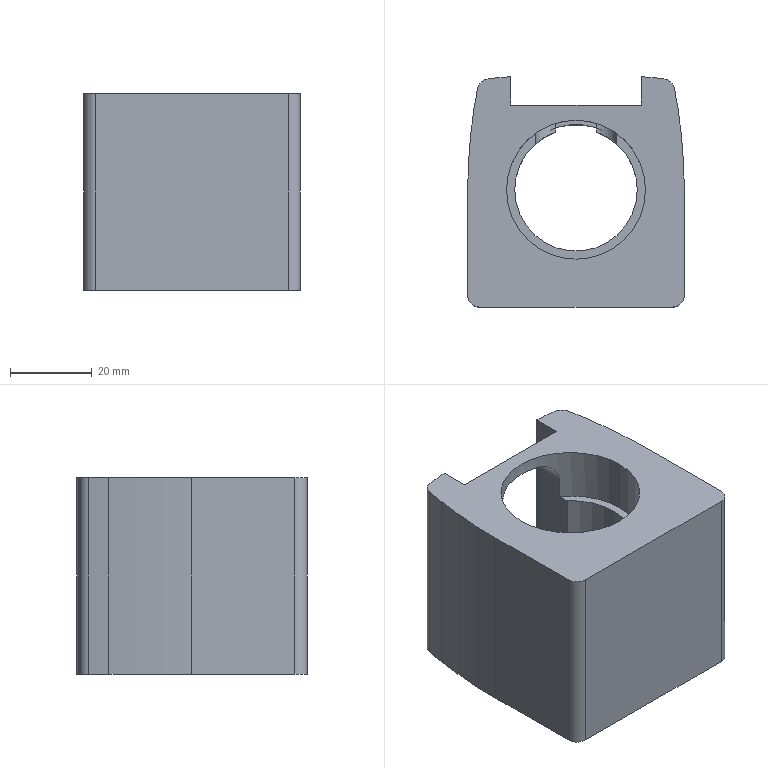Part | SolidWorks | features BaseBody 1 | 1 solid | 59 faces | box 53 x 56.359 x 48 mm | volume 87261 mm3 | cylinder 31 | plane 16 | cone 12 | commonest cylinder face diameters 2.5 x12 6 x4 10 x4 30 x3 32 x2 34 x2